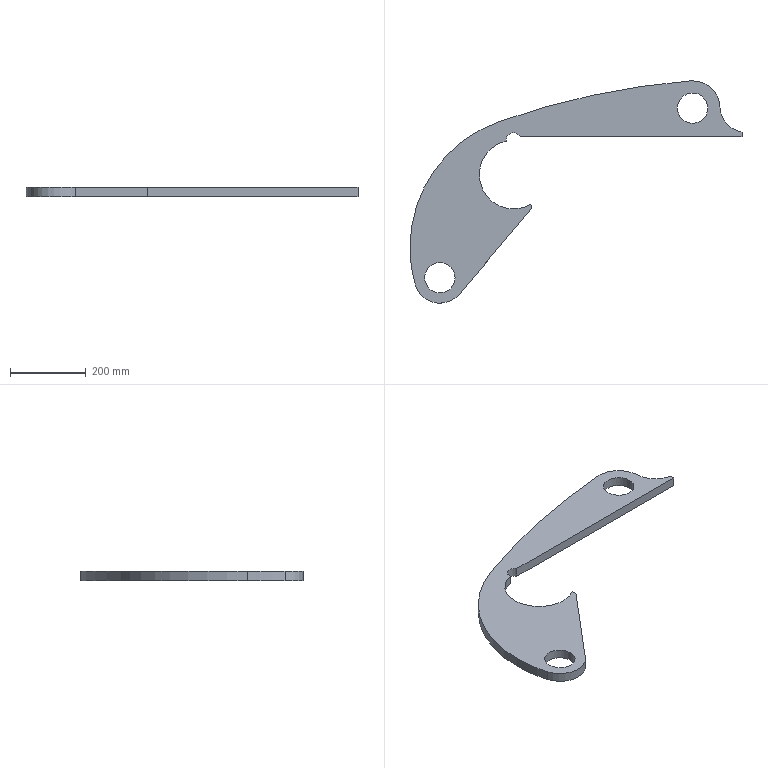Part | SolidWorks | features Extrusion 1 | 1 solid | 20 faces | box 873.891 x 585.5 x 25 mm | volume 3320222 mm3 | cylinder 14 | plane 6 | commonest cylinder face diameters 80 x4 40 x2 181 x2 700 x2 134 x1 140 x1
STEP:
#1=CARTESIAN_POINT('',(-234.2,-271.5,25.));
#2=VERTEX_POINT('',#1);
#3=CARTESIAN_POINT('',(-154.2,-271.5,25.));
#4=VERTEX_POINT('',#3);
#5=CARTESIAN_POINT('',(-194.2,-271.5,25.));
#6=DIRECTION('',(0.,0.,1.));
#7=DIRECTION('',(1.,0.,0.));
#8=AXIS2_PLACEMENT_3D('',#5,#6,#7);
#9=CIRCLE('',#8,40.);
#10=EDGE_CURVE('',#2,#4,#9,.T.);
#11=ORIENTED_EDGE('',*,*,#10,.T.);
#12=CARTESIAN_POINT('',(-154.2,-271.5,0.));
#13=VERTEX_POINT('',#12);
#14=CARTESIAN_POINT('',(-154.2,-271.5,25.));
#15=DIRECTION('',(0.,0.,-1.));
#16=VECTOR('',#15,1000.);
#17=LINE('',#14,#16);
#18=EDGE_CURVE('',#4,#13,#17,.T.);
#19=ORIENTED_EDGE('',*,*,#18,.T.);
#20=CARTESIAN_POINT('',(-234.2,-271.5,0.));
#21=VERTEX_POINT('',#20);
#22=CARTESIAN_POINT('',(-194.2,-271.5,0.));
#23=DIRECTION('',(0.,0.,1.));
#24=DIRECTION('',(1.,0.,0.));
#25=AXIS2_PLACEMENT_3D('',#22,#23,#24);
#26=CIRCLE('',#25,40.);
#27=EDGE_CURVE('',#21,#13,#26,.T.);
#28=ORIENTED_EDGE('',*,*,#27,.F.);
#29=CARTESIAN_POINT('',(-234.2,-271.5,25.));
#30=DIRECTION('',(0.,0.,-1.));
#31=VECTOR('',#30,1000.);
#32=LINE('',#29,#31);
#33=EDGE_CURVE('',#2,#21,#32,.T.);
#34=ORIENTED_EDGE('',*,*,#33,.F.);
#35=EDGE_LOOP('',(#11,#19,#28,#34));
#36=FACE_OUTER_BOUND('',#35,.T.);
#37=CARTESIAN_POINT('',(-194.2,-271.5,25.));
#38=DIRECTION('',(0.,0.,-1.));
#39=DIRECTION('',(-1.,0.,0.));
#40=AXIS2_PLACEMENT_3D('',#37,#38,#39);
#41=CYLINDRICAL_SURFACE('',#40,40.);
#42=ADVANCED_FACE('',(#36),#41,.F.);
#43=CARTESIAN_POINT('',(-19.926,88.279,25.));
#44=VERTEX_POINT('',#43);
#45=CARTESIAN_POINT('',(-90.5,0.,25.));
#46=VERTEX_POINT('',#45);
#47=CARTESIAN_POINT('',(0.,0.,25.));
#48=DIRECTION('',(0.,0.,1.));
#49=DIRECTION('',(1.,0.,0.));
#50=AXIS2_PLACEMENT_3D('',#47,#48,#49);
#51=CIRCLE('',#50,90.5);
#52=EDGE_CURVE('',#44,#46,#51,.T.);
#53=ORIENTED_EDGE('',*,*,#52,.T.);
#54=CARTESIAN_POINT('',(-90.5,0.,0.));
#55=VERTEX_POINT('',#54);
#56=CARTESIAN_POINT('',(-90.5,0.,25.));
#57=DIRECTION('',(0.,0.,-1.));
#58=VECTOR('',#57,1000.);
#59=LINE('',#56,#58);
#60=EDGE_CURVE('',#46,#55,#59,.T.);
#61=ORIENTED_EDGE('',*,*,#60,.T.);
#62=CARTESIAN_POINT('',(-19.926,88.279,0.));
#63=VERTEX_POINT('',#62);
#64=CARTESIAN_POINT('',(0.,0.,0.));
#65=DIRECTION('',(0.,0.,1.));
#66=DIRECTION('',(1.,0.,0.));
#67=AXIS2_PLACEMENT_3D('',#64,#65,#66);
#68=CIRCLE('',#67,90.5);
#69=EDGE_CURVE('',#63,#55,#68,.T.);
#70=ORIENTED_EDGE('',*,*,#69,.F.);
#71=CARTESIAN_POINT('',(-19.926,88.279,25.));
#72=DIRECTION('',(0.,0.,-1.));
#73=VECTOR('',#72,1000.);
#74=LINE('',#71,#73);
#75=EDGE_CURVE('',#44,#63,#74,.T.);
#76=ORIENTED_EDGE('',*,*,#75,.F.);
#77=EDGE_LOOP('',(#53,#61,#70,#76));
#78=FACE_OUTER_BOUND('',#77,.T.);
#79=CARTESIAN_POINT('',(0.,0.,25.));
#80=DIRECTION('',(0.,0.,-1.));
#81=DIRECTION('',(-1.,0.,0.));
#82=AXIS2_PLACEMENT_3D('',#79,#80,#81);
#83=CYLINDRICAL_SURFACE('',#82,90.5);
#84=ADVANCED_FACE('',(#78),#83,.F.);
#85=CARTESIAN_POINT('',(431.,175.,25.));
#86=VERTEX_POINT('',#85);
#87=CARTESIAN_POINT('',(511.,175.,25.));
#88=VERTEX_POINT('',#87);
#89=CARTESIAN_POINT('',(471.,175.,25.));
#90=DIRECTION('',(0.,0.,1.));
#91=DIRECTION('',(1.,0.,0.));
#92=AXIS2_PLACEMENT_3D('',#89,#90,#91);
#93=CIRCLE('',#92,40.);
#94=EDGE_CURVE('',#86,#88,#93,.T.);
#95=ORIENTED_EDGE('',*,*,#94,.T.);
#96=CARTESIAN_POINT('',(511.,175.,0.));
#97=VERTEX_POINT('',#96);
#98=CARTESIAN_POINT('',(511.,175.,25.));
#99=DIRECTION('',(0.,0.,-1.));
#100=VECTOR('',#99,1000.);
#101=LINE('',#98,#100);
#102=EDGE_CURVE('',#88,#97,#101,.T.);
#103=ORIENTED_EDGE('',*,*,#102,.T.);
#104=CARTESIAN_POINT('',(431.,175.,0.));
#105=VERTEX_POINT('',#104);
#106=CARTESIAN_POINT('',(471.,175.,0.));
#107=DIRECTION('',(0.,0.,1.));
#108=DIRECTION('',(1.,0.,0.));
#109=AXIS2_PLACEMENT_3D('',#106,#107,#108);
#110=CIRCLE('',#109,40.);
#111=EDGE_CURVE('',#105,#97,#110,.T.);
#112=ORIENTED_EDGE('',*,*,#111,.F.);
#113=CARTESIAN_POINT('',(431.,175.,25.));
#114=DIRECTION('',(0.,0.,-1.));
#115=VECTOR('',#114,1000.);
#116=LINE('',#113,#115);
#117=EDGE_CURVE('',#86,#105,#116,.T.);
#118=ORIENTED_EDGE('',*,*,#117,.F.);
#119=EDGE_LOOP('',(#95,#103,#112,#118));
#120=FACE_OUTER_BOUND('',#119,.T.);
#121=CARTESIAN_POINT('',(471.,175.,25.));
#122=DIRECTION('',(0.,0.,-1.));
#123=DIRECTION('',(-1.,0.,0.));
#124=AXIS2_PLACEMENT_3D('',#121,#122,#123);
#125=CYLINDRICAL_SURFACE('',#124,40.);
#126=ADVANCED_FACE('',(#120),#125,.F.);
#127=CARTESIAN_POINT('',(-272.891,-191.,25.));
#128=VERTEX_POINT('',#127);
#129=CARTESIAN_POINT('',(-258.432,-290.558,25.));
#130=VERTEX_POINT('',#129);
#131=CARTESIAN_POINT('',(77.109,-191.,25.));
#132=DIRECTION('',(0.,0.,1.));
#133=DIRECTION('',(1.,0.,0.));
#134=AXIS2_PLACEMENT_3D('',#131,#132,#133);
#135=CIRCLE('',#134,350.);
#136=EDGE_CURVE('',#128,#130,#135,.T.);
#137=ORIENTED_EDGE('',*,*,#136,.F.);
#138=CARTESIAN_POINT('',(-272.891,-191.,0.));
#139=VERTEX_POINT('',#138);
#140=CARTESIAN_POINT('',(-272.891,-191.,25.));
#141=DIRECTION('',(0.,0.,-1.));
#142=VECTOR('',#141,1000.);
#143=LINE('',#140,#142);
#144=EDGE_CURVE('',#128,#139,#143,.T.);
#145=ORIENTED_EDGE('',*,*,#144,.T.);
#146=CARTESIAN_POINT('',(-258.432,-290.558,0.));
#147=VERTEX_POINT('',#146);
#148=CARTESIAN_POINT('',(77.109,-191.,0.));
#149=DIRECTION('',(0.,0.,1.));
#150=DIRECTION('',(1.,0.,0.));
#151=AXIS2_PLACEMENT_3D('',#148,#149,#150);
#152=CIRCLE('',#151,350.);
#153=EDGE_CURVE('',#139,#147,#152,.T.);
#154=ORIENTED_EDGE('',*,*,#153,.T.);
#155=CARTESIAN_POINT('',(-258.432,-290.558,25.));
#156=DIRECTION('',(0.,0.,-1.));
#157=VECTOR('',#156,1000.);
#158=LINE('',#155,#157);
#159=EDGE_CURVE('',#130,#147,#158,.T.);
#160=ORIENTED_EDGE('',*,*,#159,.F.);
#161=EDGE_LOOP('',(#137,#145,#154,#160));
#162=FACE_OUTER_BOUND('',#161,.T.);
#163=CARTESIAN_POINT('',(77.109,-191.,25.));
#164=DIRECTION('',(0.,0.,-1.));
#165=DIRECTION('',(-1.,0.,0.));
#166=AXIS2_PLACEMENT_3D('',#163,#164,#165);
#167=CYLINDRICAL_SURFACE('',#166,350.);
#168=ADVANCED_FACE('',(#162),#167,.T.);
#169=CARTESIAN_POINT('',(17.321,100.,25.));
#170=VERTEX_POINT('',#169);
#171=CARTESIAN_POINT('',(-20.,90.,25.));
#172=VERTEX_POINT('',#171);
#173=CARTESIAN_POINT('',(0.,90.,25.));
#174=DIRECTION('',(0.,0.,1.));
#175=DIRECTION('',(1.,0.,0.));
#176=AXIS2_PLACEMENT_3D('',#173,#174,#175);
#177=CIRCLE('',#176,20.);
#178=EDGE_CURVE('',#170,#172,#177,.T.);
#179=ORIENTED_EDGE('',*,*,#178,.T.);
#180=CARTESIAN_POINT('',(-20.,90.,0.));
#181=VERTEX_POINT('',#180);
#182=CARTESIAN_POINT('',(-20.,90.,25.));
#183=DIRECTION('',(0.,0.,-1.));
#184=VECTOR('',#183,1000.);
#185=LINE('',#182,#184);
#186=EDGE_CURVE('',#172,#181,#185,.T.);
#187=ORIENTED_EDGE('',*,*,#186,.T.);
#188=CARTESIAN_POINT('',(17.321,100.,0.));
#189=VERTEX_POINT('',#188);
#190=CARTESIAN_POINT('',(0.,90.,0.));
#191=DIRECTION('',(0.,0.,1.));
#192=DIRECTION('',(1.,0.,0.));
#193=AXIS2_PLACEMENT_3D('',#190,#191,#192);
#194=CIRCLE('',#193,20.);
#195=EDGE_CURVE('',#189,#181,#194,.T.);
#196=ORIENTED_EDGE('',*,*,#195,.F.);
#197=CARTESIAN_POINT('',(17.321,100.,25.));
#198=DIRECTION('',(0.,0.,-1.));
#199=VECTOR('',#198,1000.);
#200=LINE('',#197,#199);
#201=EDGE_CURVE('',#170,#189,#200,.T.);
#202=ORIENTED_EDGE('',*,*,#201,.F.);
#203=EDGE_LOOP('',(#179,#187,#196,#202));
#204=FACE_OUTER_BOUND('',#203,.T.);
#205=CARTESIAN_POINT('',(0.,90.,25.));
#206=DIRECTION('',(0.,0.,-1.));
#207=DIRECTION('',(-1.,0.,0.));
#208=AXIS2_PLACEMENT_3D('',#205,#206,#207);
#209=CYLINDRICAL_SURFACE('',#208,20.);
#210=ADVANCED_FACE('',(#204),#209,.F.);
#211=ORIENTED_EDGE('',*,*,#186,.F.);
#212=CARTESIAN_POINT('',(0.,90.,25.));
#213=DIRECTION('',(0.,0.,1.));
#214=DIRECTION('',(1.,0.,0.));
#215=AXIS2_PLACEMENT_3D('',#212,#213,#214);
#216=CIRCLE('',#215,20.);
#217=EDGE_CURVE('',#172,#44,#216,.T.);
#218=ORIENTED_EDGE('',*,*,#217,.T.);
#219=ORIENTED_EDGE('',*,*,#75,.T.);
#220=CARTESIAN_POINT('',(0.,90.,0.));
#221=DIRECTION('',(0.,0.,1.));
#222=DIRECTION('',(1.,0.,0.));
#223=AXIS2_PLACEMENT_3D('',#220,#221,#222);
#224=CIRCLE('',#223,20.);
#225=EDGE_CURVE('',#181,#63,#224,.T.);
#226=ORIENTED_EDGE('',*,*,#225,.F.);
#227=EDGE_LOOP('',(#211,#218,#219,#226));
#228=FACE_OUTER_BOUND('',#227,.T.);
#229=CARTESIAN_POINT('',(0.,90.,25.));
#230=DIRECTION('',(0.,0.,-1.));
#231=DIRECTION('',(-1.,0.,0.));
#232=AXIS2_PLACEMENT_3D('',#229,#230,#231);
#233=CYLINDRICAL_SURFACE('',#232,20.);
#234=ADVANCED_FACE('',(#228),#233,.F.);
#235=CARTESIAN_POINT('',(601.,100.,0.));
#236=VERTEX_POINT('',#235);
#237=CARTESIAN_POINT('',(125.232,100.,0.));
#238=DIRECTION('',(1.,0.,0.));
#239=VECTOR('',#238,1000.);
#240=LINE('',#237,#239);
#241=EDGE_CURVE('',#189,#236,#240,.T.);
#242=ORIENTED_EDGE('',*,*,#241,.T.);
#243=CARTESIAN_POINT('',(601.,100.,25.));
#244=VERTEX_POINT('',#243);
#245=CARTESIAN_POINT('',(601.,100.,25.));
#246=DIRECTION('',(0.,0.,-1.));
#247=VECTOR('',#246,1000.);
#248=LINE('',#245,#247);
#249=EDGE_CURVE('',#244,#236,#248,.T.);
#250=ORIENTED_EDGE('',*,*,#249,.F.);
#251=CARTESIAN_POINT('',(125.232,100.,25.));
#252=DIRECTION('',(1.,0.,0.));
#253=VECTOR('',#252,1000.);
#254=LINE('',#251,#253);
#255=EDGE_CURVE('',#170,#244,#254,.T.);
#256=ORIENTED_EDGE('',*,*,#255,.F.);
#257=ORIENTED_EDGE('',*,*,#201,.T.);
#258=EDGE_LOOP('',(#242,#250,#256,#257));
#259=FACE_OUTER_BOUND('',#258,.T.);
#260=CARTESIAN_POINT('',(125.232,100.,25.));
#261=DIRECTION('',(0.,1.,0.));
#262=DIRECTION('',(0.,0.,1.));
#263=AXIS2_PLACEMENT_3D('',#260,#261,#262);
#264=PLANE('',#263);
#265=ADVANCED_FACE('',(#259),#264,.F.);
#266=CARTESIAN_POINT('',(601.,112.,0.));
#267=VERTEX_POINT('',#266);
#268=CARTESIAN_POINT('',(601.,-859.021,0.));
#269=DIRECTION('',(0.,1.,0.));
#270=VECTOR('',#269,1000.);
#271=LINE('',#268,#270);
#272=EDGE_CURVE('',#236,#267,#271,.T.);
#273=ORIENTED_EDGE('',*,*,#272,.T.);
#274=CARTESIAN_POINT('',(601.,112.,25.));
#275=VERTEX_POINT('',#274);
#276=CARTESIAN_POINT('',(601.,112.,25.));
#277=DIRECTION('',(0.,0.,-1.));
#278=VECTOR('',#277,1000.);
#279=LINE('',#276,#278);
#280=EDGE_CURVE('',#275,#267,#279,.T.);
#281=ORIENTED_EDGE('',*,*,#280,.F.);
#282=CARTESIAN_POINT('',(601.,-859.021,25.));
#283=DIRECTION('',(0.,1.,0.));
#284=VECTOR('',#283,1000.);
#285=LINE('',#282,#284);
#286=EDGE_CURVE('',#244,#275,#285,.T.);
#287=ORIENTED_EDGE('',*,*,#286,.F.);
#288=ORIENTED_EDGE('',*,*,#249,.T.);
#289=EDGE_LOOP('',(#273,#281,#287,#288));
#290=FACE_OUTER_BOUND('',#289,.T.);
#291=CARTESIAN_POINT('',(601.,-859.021,25.));
#292=DIRECTION('',(-1.,0.,0.));
#293=DIRECTION('',(0.,0.,1.));
#294=AXIS2_PLACEMENT_3D('',#291,#292,#293);
#295=PLANE('',#294);
#296=ADVANCED_FACE('',(#290),#295,.F.);
#297=CARTESIAN_POINT('',(542.936,178.035,0.));
#298=VERTEX_POINT('',#297);
#299=CARTESIAN_POINT('',(612.874,180.986,0.));
#300=DIRECTION('',(0.,0.,1.));
#301=DIRECTION('',(1.,0.,0.));
#302=AXIS2_PLACEMENT_3D('',#299,#300,#301);
#303=CIRCLE('',#302,70.);
#304=EDGE_CURVE('',#298,#267,#303,.T.);
#305=ORIENTED_EDGE('',*,*,#304,.F.);
#306=CARTESIAN_POINT('',(542.936,178.035,25.));
#307=VERTEX_POINT('',#306);
#308=CARTESIAN_POINT('',(542.936,178.035,25.));
#309=DIRECTION('',(0.,0.,-1.));
#310=VECTOR('',#309,1000.);
#311=LINE('',#308,#310);
#312=EDGE_CURVE('',#307,#298,#311,.T.);
#313=ORIENTED_EDGE('',*,*,#312,.F.);
#314=CARTESIAN_POINT('',(612.874,180.986,25.));
#315=DIRECTION('',(0.,0.,1.));
#316=DIRECTION('',(1.,0.,0.));
#317=AXIS2_PLACEMENT_3D('',#314,#315,#316);
#318=CIRCLE('',#317,70.);
#319=EDGE_CURVE('',#307,#275,#318,.T.);
#320=ORIENTED_EDGE('',*,*,#319,.T.);
#321=ORIENTED_EDGE('',*,*,#280,.T.);
#322=EDGE_LOOP('',(#305,#313,#320,#321));
#323=FACE_OUTER_BOUND('',#322,.T.);
#324=CARTESIAN_POINT('',(612.874,180.986,25.));
#325=DIRECTION('',(0.,0.,-1.));
#326=DIRECTION('',(-1.,0.,0.));
#327=AXIS2_PLACEMENT_3D('',#324,#325,#326);
#328=CYLINDRICAL_SURFACE('',#327,70.);
#329=ADVANCED_FACE('',(#323),#328,.F.);
#330=CARTESIAN_POINT('',(465.175,246.764,0.));
#331=VERTEX_POINT('',#330);
#332=CARTESIAN_POINT('',(471.,175.,0.));
#333=DIRECTION('',(0.,0.,1.));
#334=DIRECTION('',(1.,0.,0.));
#335=AXIS2_PLACEMENT_3D('',#332,#333,#334);
#336=CIRCLE('',#335,72.);
#337=EDGE_CURVE('',#298,#331,#336,.T.);
#338=ORIENTED_EDGE('',*,*,#337,.T.);
#339=CARTESIAN_POINT('',(465.175,246.764,25.));
#340=VERTEX_POINT('',#339);
#341=CARTESIAN_POINT('',(465.175,246.764,25.));
#342=DIRECTION('',(0.,0.,-1.));
#343=VECTOR('',#342,1000.);
#344=LINE('',#341,#343);
#345=EDGE_CURVE('',#340,#331,#344,.T.);
#346=ORIENTED_EDGE('',*,*,#345,.F.);
#347=CARTESIAN_POINT('',(471.,175.,25.));
#348=DIRECTION('',(0.,0.,1.));
#349=DIRECTION('',(1.,0.,0.));
#350=AXIS2_PLACEMENT_3D('',#347,#348,#349);
#351=CIRCLE('',#350,72.);
#352=EDGE_CURVE('',#307,#340,#351,.T.);
#353=ORIENTED_EDGE('',*,*,#352,.F.);
#354=ORIENTED_EDGE('',*,*,#312,.T.);
#355=EDGE_LOOP('',(#338,#346,#353,#354));
#356=FACE_OUTER_BOUND('',#355,.T.);
#357=CARTESIAN_POINT('',(471.,175.,25.));
#358=DIRECTION('',(0.,0.,-1.));
#359=DIRECTION('',(-1.,0.,0.));
#360=AXIS2_PLACEMENT_3D('',#357,#358,#359);
#361=CYLINDRICAL_SURFACE('',#360,72.);
#362=ADVANCED_FACE('',(#356),#361,.T.);
#363=CARTESIAN_POINT('',(-39.53,138.993,0.));
#364=VERTEX_POINT('',#363);
#365=CARTESIAN_POINT('',(626.982,-1746.68,0.));
#366=DIRECTION('',(0.,0.,1.));
#367=DIRECTION('',(1.,0.,0.));
#368=AXIS2_PLACEMENT_3D('',#365,#366,#367);
#369=CIRCLE('',#368,2000.);
#370=EDGE_CURVE('',#331,#364,#369,.T.);
#371=ORIENTED_EDGE('',*,*,#370,.T.);
#372=CARTESIAN_POINT('',(-39.53,138.993,25.));
#373=VERTEX_POINT('',#372);
#374=CARTESIAN_POINT('',(-39.53,138.993,25.));
#375=DIRECTION('',(0.,0.,-1.));
#376=VECTOR('',#375,1000.);
#377=LINE('',#374,#376);
#378=EDGE_CURVE('',#373,#364,#377,.T.);
#379=ORIENTED_EDGE('',*,*,#378,.F.);
#380=CARTESIAN_POINT('',(626.982,-1746.68,25.));
#381=DIRECTION('',(0.,0.,1.));
#382=DIRECTION('',(1.,0.,0.));
#383=AXIS2_PLACEMENT_3D('',#380,#381,#382);
#384=CIRCLE('',#383,2000.);
#385=EDGE_CURVE('',#340,#373,#384,.T.);
#386=ORIENTED_EDGE('',*,*,#385,.F.);
#387=ORIENTED_EDGE('',*,*,#345,.T.);
#388=EDGE_LOOP('',(#371,#379,#386,#387));
#389=FACE_OUTER_BOUND('',#388,.T.);
#390=CARTESIAN_POINT('',(626.982,-1746.68,25.));
#391=DIRECTION('',(0.,0.,-1.));
#392=DIRECTION('',(-1.,0.,0.));
#393=AXIS2_PLACEMENT_3D('',#390,#391,#392);
#394=CYLINDRICAL_SURFACE('',#393,2000.);
#395=ADVANCED_FACE('',(#389),#394,.T.);
#396=ORIENTED_EDGE('',*,*,#144,.F.);
#397=CARTESIAN_POINT('',(77.109,-191.,25.));
#398=DIRECTION('',(0.,0.,1.));
#399=DIRECTION('',(1.,0.,0.));
#400=AXIS2_PLACEMENT_3D('',#397,#398,#399);
#401=CIRCLE('',#400,350.);
#402=EDGE_CURVE('',#373,#128,#401,.T.);
#403=ORIENTED_EDGE('',*,*,#402,.F.);
#404=ORIENTED_EDGE('',*,*,#378,.T.);
#405=CARTESIAN_POINT('',(77.109,-191.,0.));
#406=DIRECTION('',(0.,0.,1.));
#407=DIRECTION('',(1.,0.,0.));
#408=AXIS2_PLACEMENT_3D('',#405,#406,#407);
#409=CIRCLE('',#408,350.);
#410=EDGE_CURVE('',#364,#139,#409,.T.);
#411=ORIENTED_EDGE('',*,*,#410,.T.);
#412=EDGE_LOOP('',(#396,#403,#404,#411));
#413=FACE_OUTER_BOUND('',#412,.T.);
#414=CARTESIAN_POINT('',(77.109,-191.,25.));
#415=DIRECTION('',(0.,0.,-1.));
#416=DIRECTION('',(-1.,0.,0.));
#417=AXIS2_PLACEMENT_3D('',#414,#415,#416);
#418=CYLINDRICAL_SURFACE('',#417,350.);
#419=ADVANCED_FACE('',(#413),#418,.T.);
#420=CARTESIAN_POINT('',(-143.033,-314.754,0.));
#421=VERTEX_POINT('',#420);
#422=CARTESIAN_POINT('',(-194.2,-271.5,0.));
#423=DIRECTION('',(0.,0.,1.));
#424=DIRECTION('',(1.,0.,0.));
#425=AXIS2_PLACEMENT_3D('',#422,#423,#424);
#426=CIRCLE('',#425,67.);
#427=EDGE_CURVE('',#147,#421,#426,.T.);
#428=ORIENTED_EDGE('',*,*,#427,.T.);
#429=CARTESIAN_POINT('',(-143.033,-314.754,25.));
#430=VERTEX_POINT('',#429);
#431=CARTESIAN_POINT('',(-143.033,-314.754,25.));
#432=DIRECTION('',(0.,0.,-1.));
#433=VECTOR('',#432,1000.);
#434=LINE('',#431,#433);
#435=EDGE_CURVE('',#430,#421,#434,.T.);
#436=ORIENTED_EDGE('',*,*,#435,.F.);
#437=CARTESIAN_POINT('',(-194.2,-271.5,25.));
#438=DIRECTION('',(0.,0.,1.));
#439=DIRECTION('',(1.,0.,0.));
#440=AXIS2_PLACEMENT_3D('',#437,#438,#439);
#441=CIRCLE('',#440,67.);
#442=EDGE_CURVE('',#130,#430,#441,.T.);
#443=ORIENTED_EDGE('',*,*,#442,.F.);
#444=ORIENTED_EDGE('',*,*,#159,.T.);
#445=EDGE_LOOP('',(#428,#436,#443,#444));
#446=FACE_OUTER_BOUND('',#445,.T.);
#447=CARTESIAN_POINT('',(-194.2,-271.5,25.));
#448=DIRECTION('',(0.,0.,-1.));
#449=DIRECTION('',(-1.,0.,0.));
#450=AXIS2_PLACEMENT_3D('',#447,#448,#449);
#451=CYLINDRICAL_SURFACE('',#450,67.);
#452=ADVANCED_FACE('',(#446),#451,.T.);
#453=CARTESIAN_POINT('',(47.3,-89.6,0.));
#454=VERTEX_POINT('',#453);
#455=CARTESIAN_POINT('',(-299.564,-499.922,0.));
#456=DIRECTION('',(-0.6456,-0.7637,0.));
#457=VECTOR('',#456,1000.);
#458=LINE('',#455,#457);
#459=EDGE_CURVE('',#454,#421,#458,.T.);
#460=ORIENTED_EDGE('',*,*,#459,.F.);
#461=CARTESIAN_POINT('',(47.3,-89.6,25.));
#462=VERTEX_POINT('',#461);
#463=CARTESIAN_POINT('',(47.3,-89.6,25.));
#464=DIRECTION('',(0.,0.,-1.));
#465=VECTOR('',#464,1000.);
#466=LINE('',#463,#465);
#467=EDGE_CURVE('',#462,#454,#466,.T.);
#468=ORIENTED_EDGE('',*,*,#467,.F.);
#469=CARTESIAN_POINT('',(-299.564,-499.922,25.));
#470=DIRECTION('',(-0.6456,-0.7637,0.));
#471=VECTOR('',#470,1000.);
#472=LINE('',#469,#471);
#473=EDGE_CURVE('',#462,#430,#472,.T.);
#474=ORIENTED_EDGE('',*,*,#473,.T.);
#475=ORIENTED_EDGE('',*,*,#435,.T.);
#476=EDGE_LOOP('',(#460,#468,#474,#475));
#477=FACE_OUTER_BOUND('',#476,.T.);
#478=CARTESIAN_POINT('',(-299.564,-499.922,25.));
#479=DIRECTION('',(0.7637,-0.6456,0.));
#480=DIRECTION('',(0.6456,0.7637,0.));
#481=AXIS2_PLACEMENT_3D('',#478,#479,#480);
#482=PLANE('',#481);
#483=ADVANCED_FACE('',(#477),#482,.T.);
#484=CARTESIAN_POINT('',(45.38,-78.3,0.));
#485=VERTEX_POINT('',#484);
#486=CARTESIAN_POINT('',(176.541,-850.304,0.));
#487=DIRECTION('',(-0.1675,0.9859,0.));
#488=VECTOR('',#487,1000.);
#489=LINE('',#486,#488);
#490=EDGE_CURVE('',#454,#485,#489,.T.);
#491=ORIENTED_EDGE('',*,*,#490,.T.);
#492=CARTESIAN_POINT('',(45.38,-78.3,25.));
#493=VERTEX_POINT('',#492);
#494=CARTESIAN_POINT('',(45.38,-78.3,25.));
#495=DIRECTION('',(0.,0.,-1.));
#496=VECTOR('',#495,1000.);
#497=LINE('',#494,#496);
#498=EDGE_CURVE('',#493,#485,#497,.T.);
#499=ORIENTED_EDGE('',*,*,#498,.F.);
#500=CARTESIAN_POINT('',(176.541,-850.304,25.));
#501=DIRECTION('',(-0.1675,0.9859,0.));
#502=VECTOR('',#501,1000.);
#503=LINE('',#500,#502);
#504=EDGE_CURVE('',#462,#493,#503,.T.);
#505=ORIENTED_EDGE('',*,*,#504,.F.);
#506=ORIENTED_EDGE('',*,*,#467,.T.);
#507=EDGE_LOOP('',(#491,#499,#505,#506));
#508=FACE_OUTER_BOUND('',#507,.T.);
#509=CARTESIAN_POINT('',(176.541,-850.304,25.));
#510=DIRECTION('',(-0.9859,-0.1675,0.));
#511=DIRECTION('',(0.1675,-0.9859,0.));
#512=AXIS2_PLACEMENT_3D('',#509,#510,#511);
#513=PLANE('',#512);
#514=ADVANCED_FACE('',(#508),#513,.F.);
#515=ORIENTED_EDGE('',*,*,#102,.F.);
#516=CARTESIAN_POINT('',(471.,175.,25.));
#517=DIRECTION('',(0.,0.,1.));
#518=DIRECTION('',(1.,0.,0.));
#519=AXIS2_PLACEMENT_3D('',#516,#517,#518);
#520=CIRCLE('',#519,40.);
#521=EDGE_CURVE('',#88,#86,#520,.T.);
#522=ORIENTED_EDGE('',*,*,#521,.T.);
#523=ORIENTED_EDGE('',*,*,#117,.T.);
#524=CARTESIAN_POINT('',(471.,175.,0.));
#525=DIRECTION('',(0.,0.,1.));
#526=DIRECTION('',(1.,0.,0.));
#527=AXIS2_PLACEMENT_3D('',#524,#525,#526);
#528=CIRCLE('',#527,40.);
#529=EDGE_CURVE('',#97,#105,#528,.T.);
#530=ORIENTED_EDGE('',*,*,#529,.F.);
#531=EDGE_LOOP('',(#515,#522,#523,#530));
#532=FACE_OUTER_BOUND('',#531,.T.);
#533=CARTESIAN_POINT('',(471.,175.,25.));
#534=DIRECTION('',(0.,0.,-1.));
#535=DIRECTION('',(-1.,0.,0.));
#536=AXIS2_PLACEMENT_3D('',#533,#534,#535);
#537=CYLINDRICAL_SURFACE('',#536,40.);
#538=ADVANCED_FACE('',(#532),#537,.F.);
#539=ORIENTED_EDGE('',*,*,#60,.F.);
#540=CARTESIAN_POINT('',(0.,0.,25.));
#541=DIRECTION('',(0.,0.,1.));
#542=DIRECTION('',(1.,0.,0.));
#543=AXIS2_PLACEMENT_3D('',#540,#541,#542);
#544=CIRCLE('',#543,90.5);
#545=EDGE_CURVE('',#46,#493,#544,.T.);
#546=ORIENTED_EDGE('',*,*,#545,.T.);
#547=ORIENTED_EDGE('',*,*,#498,.T.);
#548=CARTESIAN_POINT('',(0.,0.,0.));
#549=DIRECTION('',(0.,0.,1.));
#550=DIRECTION('',(1.,0.,0.));
#551=AXIS2_PLACEMENT_3D('',#548,#549,#550);
#552=CIRCLE('',#551,90.5);
#553=EDGE_CURVE('',#55,#485,#552,.T.);
#554=ORIENTED_EDGE('',*,*,#553,.F.);
#555=EDGE_LOOP('',(#539,#546,#547,#554));
#556=FACE_OUTER_BOUND('',#555,.T.);
#557=CARTESIAN_POINT('',(0.,0.,25.));
#558=DIRECTION('',(0.,0.,-1.));
#559=DIRECTION('',(-1.,0.,0.));
#560=AXIS2_PLACEMENT_3D('',#557,#558,#559);
#561=CYLINDRICAL_SURFACE('',#560,90.5);
#562=ADVANCED_FACE('',(#556),#561,.F.);
#563=ORIENTED_EDGE('',*,*,#18,.F.);
#564=CARTESIAN_POINT('',(-194.2,-271.5,25.));
#565=DIRECTION('',(0.,0.,1.));
#566=DIRECTION('',(1.,0.,0.));
#567=AXIS2_PLACEMENT_3D('',#564,#565,#566);
#568=CIRCLE('',#567,40.);
#569=EDGE_CURVE('',#4,#2,#568,.T.);
#570=ORIENTED_EDGE('',*,*,#569,.T.);
#571=ORIENTED_EDGE('',*,*,#33,.T.);
#572=CARTESIAN_POINT('',(-194.2,-271.5,0.));
#573=DIRECTION('',(0.,0.,1.));
#574=DIRECTION('',(1.,0.,0.));
#575=AXIS2_PLACEMENT_3D('',#572,#573,#574);
#576=CIRCLE('',#575,40.);
#577=EDGE_CURVE('',#13,#21,#576,.T.);
#578=ORIENTED_EDGE('',*,*,#577,.F.);
#579=EDGE_LOOP('',(#563,#570,#571,#578));
#580=FACE_OUTER_BOUND('',#579,.T.);
#581=CARTESIAN_POINT('',(-194.2,-271.5,25.));
#582=DIRECTION('',(0.,0.,-1.));
#583=DIRECTION('',(-1.,0.,0.));
#584=AXIS2_PLACEMENT_3D('',#581,#582,#583);
#585=CYLINDRICAL_SURFACE('',#584,40.);
#586=ADVANCED_FACE('',(#580),#585,.F.);
#587=ORIENTED_EDGE('',*,*,#178,.F.);
#588=ORIENTED_EDGE('',*,*,#255,.T.);
#589=ORIENTED_EDGE('',*,*,#286,.T.);
#590=ORIENTED_EDGE('',*,*,#319,.F.);
#591=ORIENTED_EDGE('',*,*,#352,.T.);
#592=ORIENTED_EDGE('',*,*,#385,.T.);
#593=ORIENTED_EDGE('',*,*,#402,.T.);
#594=ORIENTED_EDGE('',*,*,#136,.T.);
#595=ORIENTED_EDGE('',*,*,#442,.T.);
#596=ORIENTED_EDGE('',*,*,#473,.F.);
#597=ORIENTED_EDGE('',*,*,#504,.T.);
#598=ORIENTED_EDGE('',*,*,#545,.F.);
#599=ORIENTED_EDGE('',*,*,#52,.F.);
#600=ORIENTED_EDGE('',*,*,#217,.F.);
#601=EDGE_LOOP('',(#587,#588,#589,#590,#591,#592,#593,#594,#595,#596,#597,#598,#599,#600));
#602=FACE_OUTER_BOUND('',#601,.T.);
#603=ORIENTED_EDGE('',*,*,#94,.F.);
#604=ORIENTED_EDGE('',*,*,#521,.F.);
#605=EDGE_LOOP('',(#603,#604));
#606=FACE_BOUND('',#605,.T.);
#607=ORIENTED_EDGE('',*,*,#10,.F.);
#608=ORIENTED_EDGE('',*,*,#569,.F.);
#609=EDGE_LOOP('',(#607,#608));
#610=FACE_BOUND('',#609,.T.);
#611=CARTESIAN_POINT('',(125.232,-859.021,25.));
#612=DIRECTION('',(0.,0.,1.));
#613=DIRECTION('',(1.,0.,0.));
#614=AXIS2_PLACEMENT_3D('',#611,#612,#613);
#615=PLANE('',#614);
#616=ADVANCED_FACE('',(#602,#606,#610),#615,.T.);
#617=ORIENTED_EDGE('',*,*,#195,.T.);
#618=ORIENTED_EDGE('',*,*,#225,.T.);
#619=ORIENTED_EDGE('',*,*,#69,.T.);
#620=ORIENTED_EDGE('',*,*,#553,.T.);
#621=ORIENTED_EDGE('',*,*,#490,.F.);
#622=ORIENTED_EDGE('',*,*,#459,.T.);
#623=ORIENTED_EDGE('',*,*,#427,.F.);
#624=ORIENTED_EDGE('',*,*,#153,.F.);
#625=ORIENTED_EDGE('',*,*,#410,.F.);
#626=ORIENTED_EDGE('',*,*,#370,.F.);
#627=ORIENTED_EDGE('',*,*,#337,.F.);
#628=ORIENTED_EDGE('',*,*,#304,.T.);
#629=ORIENTED_EDGE('',*,*,#272,.F.);
#630=ORIENTED_EDGE('',*,*,#241,.F.);
#631=EDGE_LOOP('',(#617,#618,#619,#620,#621,#622,#623,#624,#625,#626,#627,#628,#629,#630));
#632=FACE_OUTER_BOUND('',#631,.T.);
#633=ORIENTED_EDGE('',*,*,#111,.T.);
#634=ORIENTED_EDGE('',*,*,#529,.T.);
#635=EDGE_LOOP('',(#633,#634));
#636=FACE_BOUND('',#635,.T.);
#637=ORIENTED_EDGE('',*,*,#27,.T.);
#638=ORIENTED_EDGE('',*,*,#577,.T.);
#639=EDGE_LOOP('',(#637,#638));
#640=FACE_BOUND('',#639,.T.);
#641=CARTESIAN_POINT('',(125.232,-859.021,0.));
#642=DIRECTION('',(0.,0.,1.));
#643=DIRECTION('',(1.,0.,0.));
#644=AXIS2_PLACEMENT_3D('',#641,#642,#643);
#645=PLANE('',#644);
#646=ADVANCED_FACE('',(#632,#636,#640),#645,.F.);
#647=CLOSED_SHELL('',(#42,#84,#126,#168,#210,#234,#265,#296,#329,#362,#395,#419,#452,#483,#514,#538,#562,#586,#616,#646));
#648=MANIFOLD_SOLID_BREP('',#647);
#649=CARTESIAN_POINT('',(0.,0.,0.));
#650=DIRECTION('',(0.,0.,1.));
#651=DIRECTION('',(1.,0.,0.));
#652=AXIS2_PLACEMENT_3D('',#649,#650,#651);
#653=(LENGTH_UNIT()NAMED_UNIT(*)SI_UNIT(.MILLI.,.METRE.));
#654=UNCERTAINTY_MEASURE_WITH_UNIT(LENGTH_MEASURE(0.00001),#653,'','');
#655=(NAMED_UNIT(*)PLANE_ANGLE_UNIT()SI_UNIT($,.RADIAN.));
#656=(NAMED_UNIT(*)SI_UNIT($,.STERADIAN.)SOLID_ANGLE_UNIT());
#657=(GEOMETRIC_REPRESENTATION_CONTEXT(3)GLOBAL_UNCERTAINTY_ASSIGNED_CONTEXT((#654))GLOBAL_UNIT_ASSIGNED_CONTEXT((#653,#655,#656))REPRESENTATION_CONTEXT('',''));
#658=ADVANCED_BREP_SHAPE_REPRESENTATION('',(#648,#652),#657);